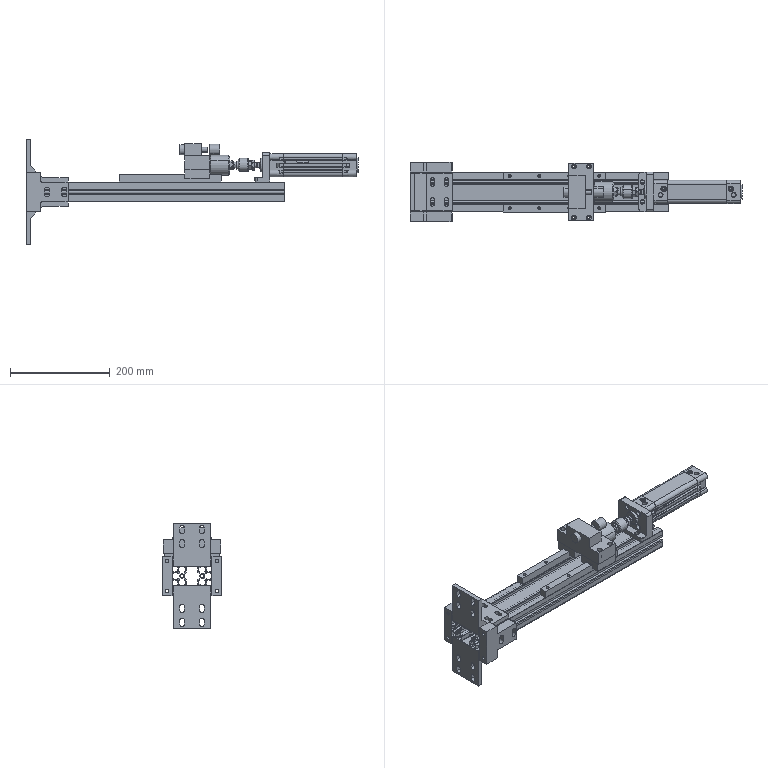Part | 25 solids | 1048 faces | box 667 x 120 x 210 mm | volume 1545625 mm3 | plane 512 | cylinder 432 | cone 98 | sphere 4 | torus 2 | commonest cylinder face diameters 1 x90 9 x54 10 x36 5 x32 6 x18 3.3 x16